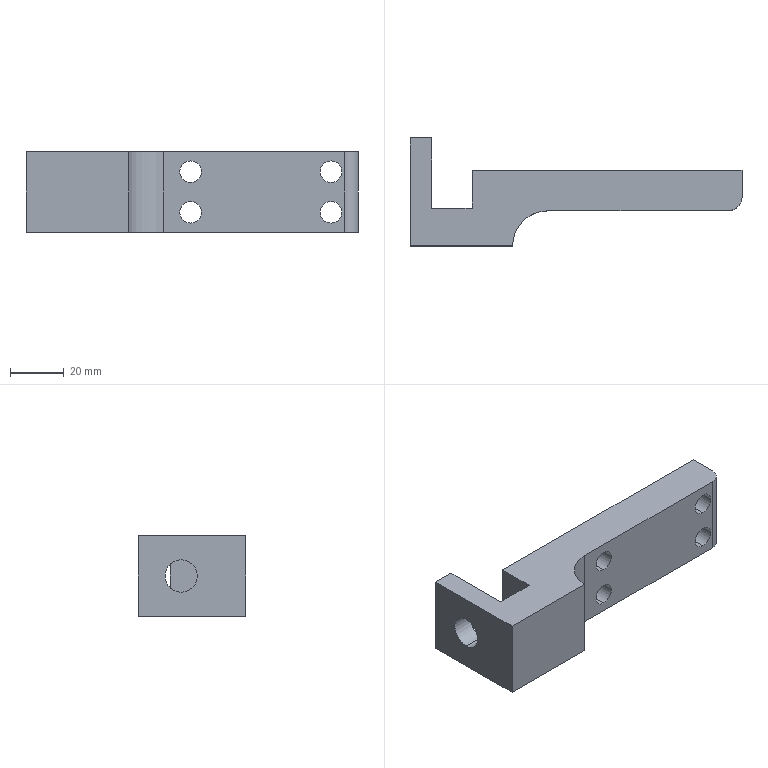Part | SolidWorks | features BaseBody 1 | 1 solid | 23 faces | box 123 x 40 x 30 mm | volume 63756 mm3 | cylinder 12 | plane 11 | commonest cylinder face diameters 8 x8 12 x2 10 x1 26 x1
STEP:
#1=CARTESIAN_POINT('',(340.,-80.,178.121));
#2=VERTEX_POINT('',#1);
#3=CARTESIAN_POINT('',(340.,-80.,186.121));
#4=VERTEX_POINT('',#3);
#5=CARTESIAN_POINT('',(340.,-80.,182.121));
#6=DIRECTION('',(0.,1.,0.));
#7=DIRECTION('',(0.,0.,-1.));
#8=AXIS2_PLACEMENT_3D('',#5,#6,#7);
#9=CIRCLE('',#8,4.);
#10=EDGE_CURVE('',#2,#4,#9,.T.);
#11=ORIENTED_EDGE('',*,*,#10,.T.);
#12=CARTESIAN_POINT('',(340.,-95.,186.121));
#13=VERTEX_POINT('',#12);
#14=CARTESIAN_POINT('',(340.,-95.,186.121));
#15=DIRECTION('',(0.,-1.,0.));
#16=VECTOR('',#15,1000.);
#17=LINE('',#14,#16);
#18=EDGE_CURVE('',#4,#13,#17,.T.);
#19=ORIENTED_EDGE('',*,*,#18,.T.);
#20=CARTESIAN_POINT('',(340.,-95.,178.121));
#21=VERTEX_POINT('',#20);
#22=CARTESIAN_POINT('',(340.,-95.,182.121));
#23=DIRECTION('',(0.,1.,0.));
#24=DIRECTION('',(0.,0.,-1.));
#25=AXIS2_PLACEMENT_3D('',#22,#23,#24);
#26=CIRCLE('',#25,4.);
#27=EDGE_CURVE('',#21,#13,#26,.T.);
#28=ORIENTED_EDGE('',*,*,#27,.F.);
#29=CARTESIAN_POINT('',(340.,-95.,178.121));
#30=DIRECTION('',(0.,-1.,0.));
#31=VECTOR('',#30,1000.);
#32=LINE('',#29,#31);
#33=EDGE_CURVE('',#2,#21,#32,.T.);
#34=ORIENTED_EDGE('',*,*,#33,.F.);
#35=EDGE_LOOP('',(#11,#19,#28,#34));
#36=FACE_OUTER_BOUND('',#35,.T.);
#37=CARTESIAN_POINT('',(340.,-95.,182.121));
#38=DIRECTION('',(0.,-1.,0.));
#39=DIRECTION('',(0.,0.,-1.));
#40=AXIS2_PLACEMENT_3D('',#37,#38,#39);
#41=CYLINDRICAL_SURFACE('',#40,4.);
#42=ADVANCED_FACE('',(#36),#41,.F.);
#43=CARTESIAN_POINT('',(340.,-80.,193.121));
#44=VERTEX_POINT('',#43);
#45=CARTESIAN_POINT('',(340.,-80.,201.121));
#46=VERTEX_POINT('',#45);
#47=CARTESIAN_POINT('',(340.,-80.,197.121));
#48=DIRECTION('',(0.,1.,0.));
#49=DIRECTION('',(0.,0.,-1.));
#50=AXIS2_PLACEMENT_3D('',#47,#48,#49);
#51=CIRCLE('',#50,4.);
#52=EDGE_CURVE('',#44,#46,#51,.T.);
#53=ORIENTED_EDGE('',*,*,#52,.T.);
#54=CARTESIAN_POINT('',(340.,-95.,201.121));
#55=VERTEX_POINT('',#54);
#56=CARTESIAN_POINT('',(340.,-95.,201.121));
#57=DIRECTION('',(0.,-1.,0.));
#58=VECTOR('',#57,1000.);
#59=LINE('',#56,#58);
#60=EDGE_CURVE('',#46,#55,#59,.T.);
#61=ORIENTED_EDGE('',*,*,#60,.T.);
#62=CARTESIAN_POINT('',(340.,-95.,193.121));
#63=VERTEX_POINT('',#62);
#64=CARTESIAN_POINT('',(340.,-95.,197.121));
#65=DIRECTION('',(0.,1.,0.));
#66=DIRECTION('',(0.,0.,-1.));
#67=AXIS2_PLACEMENT_3D('',#64,#65,#66);
#68=CIRCLE('',#67,4.);
#69=EDGE_CURVE('',#63,#55,#68,.T.);
#70=ORIENTED_EDGE('',*,*,#69,.F.);
#71=CARTESIAN_POINT('',(340.,-95.,193.121));
#72=DIRECTION('',(0.,-1.,0.));
#73=VECTOR('',#72,1000.);
#74=LINE('',#71,#73);
#75=EDGE_CURVE('',#44,#63,#74,.T.);
#76=ORIENTED_EDGE('',*,*,#75,.F.);
#77=EDGE_LOOP('',(#53,#61,#70,#76));
#78=FACE_OUTER_BOUND('',#77,.T.);
#79=CARTESIAN_POINT('',(340.,-95.,197.121));
#80=DIRECTION('',(0.,-1.,0.));
#81=DIRECTION('',(0.,0.,-1.));
#82=AXIS2_PLACEMENT_3D('',#79,#80,#81);
#83=CYLINDRICAL_SURFACE('',#82,4.);
#84=ADVANCED_FACE('',(#78),#83,.F.);
#85=CARTESIAN_POINT('',(288.,-80.,193.121));
#86=VERTEX_POINT('',#85);
#87=CARTESIAN_POINT('',(288.,-80.,201.121));
#88=VERTEX_POINT('',#87);
#89=CARTESIAN_POINT('',(288.,-80.,197.121));
#90=DIRECTION('',(0.,1.,0.));
#91=DIRECTION('',(0.,0.,-1.));
#92=AXIS2_PLACEMENT_3D('',#89,#90,#91);
#93=CIRCLE('',#92,4.);
#94=EDGE_CURVE('',#86,#88,#93,.T.);
#95=ORIENTED_EDGE('',*,*,#94,.T.);
#96=CARTESIAN_POINT('',(288.,-95.,201.121));
#97=VERTEX_POINT('',#96);
#98=CARTESIAN_POINT('',(288.,-95.,201.121));
#99=DIRECTION('',(0.,-1.,0.));
#100=VECTOR('',#99,1000.);
#101=LINE('',#98,#100);
#102=EDGE_CURVE('',#88,#97,#101,.T.);
#103=ORIENTED_EDGE('',*,*,#102,.T.);
#104=CARTESIAN_POINT('',(288.,-95.,193.121));
#105=VERTEX_POINT('',#104);
#106=CARTESIAN_POINT('',(288.,-95.,197.121));
#107=DIRECTION('',(0.,1.,0.));
#108=DIRECTION('',(0.,0.,-1.));
#109=AXIS2_PLACEMENT_3D('',#106,#107,#108);
#110=CIRCLE('',#109,4.);
#111=EDGE_CURVE('',#105,#97,#110,.T.);
#112=ORIENTED_EDGE('',*,*,#111,.F.);
#113=CARTESIAN_POINT('',(288.,-95.,193.121));
#114=DIRECTION('',(0.,-1.,0.));
#115=VECTOR('',#114,1000.);
#116=LINE('',#113,#115);
#117=EDGE_CURVE('',#86,#105,#116,.T.);
#118=ORIENTED_EDGE('',*,*,#117,.F.);
#119=EDGE_LOOP('',(#95,#103,#112,#118));
#120=FACE_OUTER_BOUND('',#119,.T.);
#121=CARTESIAN_POINT('',(288.,-95.,197.121));
#122=DIRECTION('',(0.,-1.,0.));
#123=DIRECTION('',(0.,0.,-1.));
#124=AXIS2_PLACEMENT_3D('',#121,#122,#123);
#125=CYLINDRICAL_SURFACE('',#124,4.);
#126=ADVANCED_FACE('',(#120),#125,.F.);
#127=CARTESIAN_POINT('',(288.,-80.,178.121));
#128=VERTEX_POINT('',#127);
#129=CARTESIAN_POINT('',(288.,-80.,186.121));
#130=VERTEX_POINT('',#129);
#131=CARTESIAN_POINT('',(288.,-80.,182.121));
#132=DIRECTION('',(0.,1.,0.));
#133=DIRECTION('',(0.,0.,-1.));
#134=AXIS2_PLACEMENT_3D('',#131,#132,#133);
#135=CIRCLE('',#134,4.);
#136=EDGE_CURVE('',#128,#130,#135,.T.);
#137=ORIENTED_EDGE('',*,*,#136,.T.);
#138=CARTESIAN_POINT('',(288.,-95.,186.121));
#139=VERTEX_POINT('',#138);
#140=CARTESIAN_POINT('',(288.,-95.,186.121));
#141=DIRECTION('',(0.,-1.,0.));
#142=VECTOR('',#141,1000.);
#143=LINE('',#140,#142);
#144=EDGE_CURVE('',#130,#139,#143,.T.);
#145=ORIENTED_EDGE('',*,*,#144,.T.);
#146=CARTESIAN_POINT('',(288.,-95.,178.121));
#147=VERTEX_POINT('',#146);
#148=CARTESIAN_POINT('',(288.,-95.,182.121));
#149=DIRECTION('',(0.,1.,0.));
#150=DIRECTION('',(0.,0.,-1.));
#151=AXIS2_PLACEMENT_3D('',#148,#149,#150);
#152=CIRCLE('',#151,4.);
#153=EDGE_CURVE('',#147,#139,#152,.T.);
#154=ORIENTED_EDGE('',*,*,#153,.F.);
#155=CARTESIAN_POINT('',(288.,-95.,178.121));
#156=DIRECTION('',(0.,-1.,0.));
#157=VECTOR('',#156,1000.);
#158=LINE('',#155,#157);
#159=EDGE_CURVE('',#128,#147,#158,.T.);
#160=ORIENTED_EDGE('',*,*,#159,.F.);
#161=EDGE_LOOP('',(#137,#145,#154,#160));
#162=FACE_OUTER_BOUND('',#161,.T.);
#163=CARTESIAN_POINT('',(288.,-95.,182.121));
#164=DIRECTION('',(0.,-1.,0.));
#165=DIRECTION('',(0.,0.,-1.));
#166=AXIS2_PLACEMENT_3D('',#163,#164,#165);
#167=CYLINDRICAL_SURFACE('',#166,4.);
#168=ADVANCED_FACE('',(#162),#167,.F.);
#169=CARTESIAN_POINT('',(235.,-84.,195.621));
#170=VERTEX_POINT('',#169);
#171=CARTESIAN_POINT('',(235.,-84.,183.621));
#172=VERTEX_POINT('',#171);
#173=CARTESIAN_POINT('',(235.,-84.,189.621));
#174=DIRECTION('',(1.,0.,0.));
#175=DIRECTION('',(0.,0.,1.));
#176=AXIS2_PLACEMENT_3D('',#173,#174,#175);
#177=CIRCLE('',#176,6.);
#178=EDGE_CURVE('',#170,#172,#177,.T.);
#179=ORIENTED_EDGE('',*,*,#178,.T.);
#180=CARTESIAN_POINT('',(227.,-84.,183.621));
#181=VERTEX_POINT('',#180);
#182=CARTESIAN_POINT('',(251.971,-84.,183.621));
#183=DIRECTION('',(-1.,0.,0.));
#184=VECTOR('',#183,1000.);
#185=LINE('',#182,#184);
#186=EDGE_CURVE('',#172,#181,#185,.T.);
#187=ORIENTED_EDGE('',*,*,#186,.T.);
#188=CARTESIAN_POINT('',(227.,-84.,195.621));
#189=VERTEX_POINT('',#188);
#190=CARTESIAN_POINT('',(227.,-84.,189.621));
#191=DIRECTION('',(-1.,0.,0.));
#192=DIRECTION('',(0.,0.,1.));
#193=AXIS2_PLACEMENT_3D('',#190,#191,#192);
#194=CIRCLE('',#193,6.);
#195=EDGE_CURVE('',#181,#189,#194,.T.);
#196=ORIENTED_EDGE('',*,*,#195,.T.);
#197=CARTESIAN_POINT('',(251.971,-84.,195.621));
#198=DIRECTION('',(-1.,0.,0.));
#199=VECTOR('',#198,1000.);
#200=LINE('',#197,#199);
#201=EDGE_CURVE('',#170,#189,#200,.T.);
#202=ORIENTED_EDGE('',*,*,#201,.F.);
#203=EDGE_LOOP('',(#179,#187,#196,#202));
#204=FACE_OUTER_BOUND('',#203,.T.);
#205=CARTESIAN_POINT('',(251.971,-84.,189.621));
#206=DIRECTION('',(-1.,0.,0.));
#207=DIRECTION('',(0.,0.,1.));
#208=AXIS2_PLACEMENT_3D('',#205,#206,#207);
#209=CYLINDRICAL_SURFACE('',#208,6.);
#210=ADVANCED_FACE('',(#204),#209,.F.);
#211=CARTESIAN_POINT('',(350.,-80.,174.621));
#212=VERTEX_POINT('',#211);
#213=CARTESIAN_POINT('',(350.,-80.,204.621));
#214=VERTEX_POINT('',#213);
#215=CARTESIAN_POINT('',(350.,-80.,174.621));
#216=DIRECTION('',(0.,0.,1.));
#217=VECTOR('',#216,1000.);
#218=LINE('',#215,#217);
#219=EDGE_CURVE('',#212,#214,#218,.T.);
#220=ORIENTED_EDGE('',*,*,#219,.F.);
#221=CARTESIAN_POINT('',(250.,-80.,174.621));
#222=VERTEX_POINT('',#221);
#223=CARTESIAN_POINT('',(350.,-80.,174.621));
#224=DIRECTION('',(1.,0.,0.));
#225=VECTOR('',#224,1000.);
#226=LINE('',#223,#225);
#227=EDGE_CURVE('',#222,#212,#226,.T.);
#228=ORIENTED_EDGE('',*,*,#227,.F.);
#229=CARTESIAN_POINT('',(250.,-80.,204.621));
#230=VERTEX_POINT('',#229);
#231=CARTESIAN_POINT('',(250.,-80.,174.621));
#232=DIRECTION('',(0.,0.,-1.));
#233=VECTOR('',#232,1000.);
#234=LINE('',#231,#233);
#235=EDGE_CURVE('',#230,#222,#234,.T.);
#236=ORIENTED_EDGE('',*,*,#235,.F.);
#237=CARTESIAN_POINT('',(350.,-80.,204.621));
#238=DIRECTION('',(-1.,0.,0.));
#239=VECTOR('',#238,1000.);
#240=LINE('',#237,#239);
#241=EDGE_CURVE('',#214,#230,#240,.T.);
#242=ORIENTED_EDGE('',*,*,#241,.F.);
#243=EDGE_LOOP('',(#220,#228,#236,#242));
#244=FACE_OUTER_BOUND('',#243,.T.);
#245=ORIENTED_EDGE('',*,*,#10,.F.);
#246=CARTESIAN_POINT('',(340.,-80.,182.121));
#247=DIRECTION('',(0.,1.,0.));
#248=DIRECTION('',(0.,0.,-1.));
#249=AXIS2_PLACEMENT_3D('',#246,#247,#248);
#250=CIRCLE('',#249,4.);
#251=EDGE_CURVE('',#4,#2,#250,.T.);
#252=ORIENTED_EDGE('',*,*,#251,.F.);
#253=EDGE_LOOP('',(#245,#252));
#254=FACE_BOUND('',#253,.T.);
#255=ORIENTED_EDGE('',*,*,#52,.F.);
#256=CARTESIAN_POINT('',(340.,-80.,197.121));
#257=DIRECTION('',(0.,1.,0.));
#258=DIRECTION('',(0.,0.,-1.));
#259=AXIS2_PLACEMENT_3D('',#256,#257,#258);
#260=CIRCLE('',#259,4.);
#261=EDGE_CURVE('',#46,#44,#260,.T.);
#262=ORIENTED_EDGE('',*,*,#261,.F.);
#263=EDGE_LOOP('',(#255,#262));
#264=FACE_BOUND('',#263,.T.);
#265=ORIENTED_EDGE('',*,*,#94,.F.);
#266=CARTESIAN_POINT('',(288.,-80.,197.121));
#267=DIRECTION('',(0.,1.,0.));
#268=DIRECTION('',(0.,0.,-1.));
#269=AXIS2_PLACEMENT_3D('',#266,#267,#268);
#270=CIRCLE('',#269,4.);
#271=EDGE_CURVE('',#88,#86,#270,.T.);
#272=ORIENTED_EDGE('',*,*,#271,.F.);
#273=EDGE_LOOP('',(#265,#272));
#274=FACE_BOUND('',#273,.T.);
#275=ORIENTED_EDGE('',*,*,#136,.F.);
#276=CARTESIAN_POINT('',(288.,-80.,182.121));
#277=DIRECTION('',(0.,1.,0.));
#278=DIRECTION('',(0.,0.,-1.));
#279=AXIS2_PLACEMENT_3D('',#276,#277,#278);
#280=CIRCLE('',#279,4.);
#281=EDGE_CURVE('',#130,#128,#280,.T.);
#282=ORIENTED_EDGE('',*,*,#281,.F.);
#283=EDGE_LOOP('',(#275,#282));
#284=FACE_BOUND('',#283,.T.);
#285=CARTESIAN_POINT('',(350.,-80.,174.621));
#286=DIRECTION('',(0.,-1.,0.));
#287=DIRECTION('',(0.,0.,-1.));
#288=AXIS2_PLACEMENT_3D('',#285,#286,#287);
#289=PLANE('',#288);
#290=ADVANCED_FACE('',(#244,#254,#264,#274,#284),#289,.F.);
#291=CARTESIAN_POINT('',(350.,-90.,204.621));
#292=VERTEX_POINT('',#291);
#293=CARTESIAN_POINT('',(345.,-95.,204.621));
#294=VERTEX_POINT('',#293);
#295=CARTESIAN_POINT('',(345.,-90.,204.621));
#296=DIRECTION('',(0.,0.,-1.));
#297=DIRECTION('',(1.,0.,0.));
#298=AXIS2_PLACEMENT_3D('',#295,#296,#297);
#299=CIRCLE('',#298,5.);
#300=EDGE_CURVE('',#292,#294,#299,.T.);
#301=ORIENTED_EDGE('',*,*,#300,.F.);
#302=CARTESIAN_POINT('',(350.,-82.6,204.621));
#303=DIRECTION('',(0.,-1.,0.));
#304=VECTOR('',#303,1000.);
#305=LINE('',#302,#304);
#306=EDGE_CURVE('',#214,#292,#305,.T.);
#307=ORIENTED_EDGE('',*,*,#306,.F.);
#308=ORIENTED_EDGE('',*,*,#241,.T.);
#309=CARTESIAN_POINT('',(250.,-94.,204.621));
#310=VERTEX_POINT('',#309);
#311=CARTESIAN_POINT('',(250.,-82.6,204.621));
#312=DIRECTION('',(0.,1.,0.));
#313=VECTOR('',#312,1000.);
#314=LINE('',#311,#313);
#315=EDGE_CURVE('',#310,#230,#314,.T.);
#316=ORIENTED_EDGE('',*,*,#315,.F.);
#317=CARTESIAN_POINT('',(235.,-94.,204.621));
#318=VERTEX_POINT('',#317);
#319=CARTESIAN_POINT('',(251.867,-94.,204.621));
#320=DIRECTION('',(1.,0.,0.));
#321=VECTOR('',#320,1000.);
#322=LINE('',#319,#321);
#323=EDGE_CURVE('',#318,#310,#322,.T.);
#324=ORIENTED_EDGE('',*,*,#323,.F.);
#325=CARTESIAN_POINT('',(235.,-68.,204.621));
#326=VERTEX_POINT('',#325);
#327=CARTESIAN_POINT('',(235.,-82.6,204.621));
#328=DIRECTION('',(0.,-1.,0.));
#329=VECTOR('',#328,1000.);
#330=LINE('',#327,#329);
#331=EDGE_CURVE('',#326,#318,#330,.T.);
#332=ORIENTED_EDGE('',*,*,#331,.F.);
#333=CARTESIAN_POINT('',(227.,-68.,204.621));
#334=VERTEX_POINT('',#333);
#335=CARTESIAN_POINT('',(251.867,-68.,204.621));
#336=DIRECTION('',(1.,0.,0.));
#337=VECTOR('',#336,1000.);
#338=LINE('',#335,#337);
#339=EDGE_CURVE('',#334,#326,#338,.T.);
#340=ORIENTED_EDGE('',*,*,#339,.F.);
#341=CARTESIAN_POINT('',(227.,-108.,204.621));
#342=VERTEX_POINT('',#341);
#343=CARTESIAN_POINT('',(227.,-82.6,204.621));
#344=DIRECTION('',(0.,1.,0.));
#345=VECTOR('',#344,1000.);
#346=LINE('',#343,#345);
#347=EDGE_CURVE('',#342,#334,#346,.T.);
#348=ORIENTED_EDGE('',*,*,#347,.F.);
#349=CARTESIAN_POINT('',(265.,-108.,204.621));
#350=VERTEX_POINT('',#349);
#351=CARTESIAN_POINT('',(251.867,-108.,204.621));
#352=DIRECTION('',(-1.,0.,0.));
#353=VECTOR('',#352,1000.);
#354=LINE('',#351,#353);
#355=EDGE_CURVE('',#350,#342,#354,.T.);
#356=ORIENTED_EDGE('',*,*,#355,.F.);
#357=CARTESIAN_POINT('',(278.,-95.,204.621));
#358=VERTEX_POINT('',#357);
#359=CARTESIAN_POINT('',(278.,-108.,204.621));
#360=DIRECTION('',(0.,0.,1.));
#361=DIRECTION('',(-1.,0.,0.));
#362=AXIS2_PLACEMENT_3D('',#359,#360,#361);
#363=CIRCLE('',#362,13.);
#364=EDGE_CURVE('',#358,#350,#363,.T.);
#365=ORIENTED_EDGE('',*,*,#364,.F.);
#366=CARTESIAN_POINT('',(251.867,-95.,204.621));
#367=DIRECTION('',(-1.,0.,0.));
#368=VECTOR('',#367,1000.);
#369=LINE('',#366,#368);
#370=EDGE_CURVE('',#294,#358,#369,.T.);
#371=ORIENTED_EDGE('',*,*,#370,.F.);
#372=EDGE_LOOP('',(#301,#307,#308,#316,#324,#332,#340,#348,#356,#365,#371));
#373=FACE_OUTER_BOUND('',#372,.T.);
#374=CARTESIAN_POINT('',(251.867,-82.6,204.621));
#375=DIRECTION('',(0.,0.,-1.));
#376=DIRECTION('',(-1.,0.,0.));
#377=AXIS2_PLACEMENT_3D('',#374,#375,#376);
#378=PLANE('',#377);
#379=ADVANCED_FACE('',(#373),#378,.F.);
#380=CARTESIAN_POINT('',(350.,-90.,174.621));
#381=VERTEX_POINT('',#380);
#382=CARTESIAN_POINT('',(350.,-90.,174.621));
#383=DIRECTION('',(0.,0.,1.));
#384=VECTOR('',#383,1000.);
#385=LINE('',#382,#384);
#386=EDGE_CURVE('',#381,#292,#385,.T.);
#387=ORIENTED_EDGE('',*,*,#386,.F.);
#388=CARTESIAN_POINT('',(350.,-80.,174.621));
#389=DIRECTION('',(0.,-1.,0.));
#390=VECTOR('',#389,1000.);
#391=LINE('',#388,#390);
#392=EDGE_CURVE('',#212,#381,#391,.T.);
#393=ORIENTED_EDGE('',*,*,#392,.F.);
#394=ORIENTED_EDGE('',*,*,#219,.T.);
#395=ORIENTED_EDGE('',*,*,#306,.T.);
#396=EDGE_LOOP('',(#387,#393,#394,#395));
#397=FACE_OUTER_BOUND('',#396,.T.);
#398=CARTESIAN_POINT('',(350.,-80.,174.621));
#399=DIRECTION('',(-1.,0.,0.));
#400=DIRECTION('',(0.,0.,1.));
#401=AXIS2_PLACEMENT_3D('',#398,#399,#400);
#402=PLANE('',#401);
#403=ADVANCED_FACE('',(#397),#402,.F.);
#404=CARTESIAN_POINT('',(250.,-94.,174.621));
#405=VERTEX_POINT('',#404);
#406=CARTESIAN_POINT('',(250.,-82.6,174.621));
#407=DIRECTION('',(0.,1.,0.));
#408=VECTOR('',#407,1000.);
#409=LINE('',#406,#408);
#410=EDGE_CURVE('',#405,#222,#409,.T.);
#411=ORIENTED_EDGE('',*,*,#410,.T.);
#412=ORIENTED_EDGE('',*,*,#227,.T.);
#413=ORIENTED_EDGE('',*,*,#392,.T.);
#414=CARTESIAN_POINT('',(345.,-95.,174.621));
#415=VERTEX_POINT('',#414);
#416=CARTESIAN_POINT('',(345.,-90.,174.621));
#417=DIRECTION('',(0.,0.,-1.));
#418=DIRECTION('',(1.,0.,0.));
#419=AXIS2_PLACEMENT_3D('',#416,#417,#418);
#420=CIRCLE('',#419,5.);
#421=EDGE_CURVE('',#381,#415,#420,.T.);
#422=ORIENTED_EDGE('',*,*,#421,.T.);
#423=CARTESIAN_POINT('',(278.,-95.,174.621));
#424=VERTEX_POINT('',#423);
#425=CARTESIAN_POINT('',(251.867,-95.,174.621));
#426=DIRECTION('',(-1.,0.,0.));
#427=VECTOR('',#426,1000.);
#428=LINE('',#425,#427);
#429=EDGE_CURVE('',#415,#424,#428,.T.);
#430=ORIENTED_EDGE('',*,*,#429,.T.);
#431=CARTESIAN_POINT('',(265.,-108.,174.621));
#432=VERTEX_POINT('',#431);
#433=CARTESIAN_POINT('',(278.,-108.,174.621));
#434=DIRECTION('',(0.,0.,1.));
#435=DIRECTION('',(-1.,0.,0.));
#436=AXIS2_PLACEMENT_3D('',#433,#434,#435);
#437=CIRCLE('',#436,13.);
#438=EDGE_CURVE('',#424,#432,#437,.T.);
#439=ORIENTED_EDGE('',*,*,#438,.T.);
#440=CARTESIAN_POINT('',(227.,-108.,174.621));
#441=VERTEX_POINT('',#440);
#442=CARTESIAN_POINT('',(251.867,-108.,174.621));
#443=DIRECTION('',(-1.,0.,0.));
#444=VECTOR('',#443,1000.);
#445=LINE('',#442,#444);
#446=EDGE_CURVE('',#432,#441,#445,.T.);
#447=ORIENTED_EDGE('',*,*,#446,.T.);
#448=CARTESIAN_POINT('',(227.,-68.,174.621));
#449=VERTEX_POINT('',#448);
#450=CARTESIAN_POINT('',(227.,-82.6,174.621));
#451=DIRECTION('',(0.,1.,0.));
#452=VECTOR('',#451,1000.);
#453=LINE('',#450,#452);
#454=EDGE_CURVE('',#441,#449,#453,.T.);
#455=ORIENTED_EDGE('',*,*,#454,.T.);
#456=CARTESIAN_POINT('',(235.,-68.,174.621));
#457=VERTEX_POINT('',#456);
#458=CARTESIAN_POINT('',(251.867,-68.,174.621));
#459=DIRECTION('',(1.,0.,0.));
#460=VECTOR('',#459,1000.);
#461=LINE('',#458,#460);
#462=EDGE_CURVE('',#449,#457,#461,.T.);
#463=ORIENTED_EDGE('',*,*,#462,.T.);
#464=CARTESIAN_POINT('',(235.,-94.,174.621));
#465=VERTEX_POINT('',#464);
#466=CARTESIAN_POINT('',(235.,-82.6,174.621));
#467=DIRECTION('',(0.,-1.,0.));
#468=VECTOR('',#467,1000.);
#469=LINE('',#466,#468);
#470=EDGE_CURVE('',#457,#465,#469,.T.);
#471=ORIENTED_EDGE('',*,*,#470,.T.);
#472=CARTESIAN_POINT('',(251.867,-94.,174.621));
#473=DIRECTION('',(1.,0.,0.));
#474=VECTOR('',#473,1000.);
#475=LINE('',#472,#474);
#476=EDGE_CURVE('',#465,#405,#475,.T.);
#477=ORIENTED_EDGE('',*,*,#476,.T.);
#478=EDGE_LOOP('',(#411,#412,#413,#422,#430,#439,#447,#455,#463,#471,#477));
#479=FACE_OUTER_BOUND('',#478,.T.);
#480=CARTESIAN_POINT('',(251.867,-82.6,174.621));
#481=DIRECTION('',(0.,0.,-1.));
#482=DIRECTION('',(-1.,0.,0.));
#483=AXIS2_PLACEMENT_3D('',#480,#481,#482);
#484=PLANE('',#483);
#485=ADVANCED_FACE('',(#479),#484,.T.);
#486=ORIENTED_EDGE('',*,*,#235,.T.);
#487=ORIENTED_EDGE('',*,*,#410,.F.);
#488=CARTESIAN_POINT('',(250.,-94.,174.621));
#489=DIRECTION('',(0.,0.,-1.));
#490=VECTOR('',#489,1000.);
#491=LINE('',#488,#490);
#492=EDGE_CURVE('',#310,#405,#491,.T.);
#493=ORIENTED_EDGE('',*,*,#492,.F.);
#494=ORIENTED_EDGE('',*,*,#315,.T.);
#495=EDGE_LOOP('',(#486,#487,#493,#494));
#496=FACE_OUTER_BOUND('',#495,.T.);
#497=CARTESIAN_POINT('',(250.,-80.,174.621));
#498=DIRECTION('',(1.,0.,0.));
#499=DIRECTION('',(0.,0.,-1.));
#500=AXIS2_PLACEMENT_3D('',#497,#498,#499);
#501=PLANE('',#500);
#502=ADVANCED_FACE('',(#496),#501,.F.);
#503=ORIENTED_EDGE('',*,*,#18,.F.);
#504=ORIENTED_EDGE('',*,*,#251,.T.);
#505=ORIENTED_EDGE('',*,*,#33,.T.);
#506=CARTESIAN_POINT('',(340.,-95.,182.121));
#507=DIRECTION('',(0.,1.,0.));
#508=DIRECTION('',(0.,0.,-1.));
#509=AXIS2_PLACEMENT_3D('',#506,#507,#508);
#510=CIRCLE('',#509,4.);
#511=EDGE_CURVE('',#13,#21,#510,.T.);
#512=ORIENTED_EDGE('',*,*,#511,.F.);
#513=EDGE_LOOP('',(#503,#504,#505,#512));
#514=FACE_OUTER_BOUND('',#513,.T.);
#515=CARTESIAN_POINT('',(340.,-95.,182.121));
#516=DIRECTION('',(0.,-1.,0.));
#517=DIRECTION('',(0.,0.,-1.));
#518=AXIS2_PLACEMENT_3D('',#515,#516,#517);
#519=CYLINDRICAL_SURFACE('',#518,4.);
#520=ADVANCED_FACE('',(#514),#519,.F.);
#521=ORIENTED_EDGE('',*,*,#60,.F.);
#522=ORIENTED_EDGE('',*,*,#261,.T.);
#523=ORIENTED_EDGE('',*,*,#75,.T.);
#524=CARTESIAN_POINT('',(340.,-95.,197.121));
#525=DIRECTION('',(0.,1.,0.));
#526=DIRECTION('',(0.,0.,-1.));
#527=AXIS2_PLACEMENT_3D('',#524,#525,#526);
#528=CIRCLE('',#527,4.);
#529=EDGE_CURVE('',#55,#63,#528,.T.);
#530=ORIENTED_EDGE('',*,*,#529,.F.);
#531=EDGE_LOOP('',(#521,#522,#523,#530));
#532=FACE_OUTER_BOUND('',#531,.T.);
#533=CARTESIAN_POINT('',(340.,-95.,197.121));
#534=DIRECTION('',(0.,-1.,0.));
#535=DIRECTION('',(0.,0.,-1.));
#536=AXIS2_PLACEMENT_3D('',#533,#534,#535);
#537=CYLINDRICAL_SURFACE('',#536,4.);
#538=ADVANCED_FACE('',(#532),#537,.F.);
#539=ORIENTED_EDGE('',*,*,#102,.F.);
#540=ORIENTED_EDGE('',*,*,#271,.T.);
#541=ORIENTED_EDGE('',*,*,#117,.T.);
#542=CARTESIAN_POINT('',(288.,-95.,197.121));
#543=DIRECTION('',(0.,1.,0.));
#544=DIRECTION('',(0.,0.,-1.));
#545=AXIS2_PLACEMENT_3D('',#542,#543,#544);
#546=CIRCLE('',#545,4.);
#547=EDGE_CURVE('',#97,#105,#546,.T.);
#548=ORIENTED_EDGE('',*,*,#547,.F.);
#549=EDGE_LOOP('',(#539,#540,#541,#548));
#550=FACE_OUTER_BOUND('',#549,.T.);
#551=CARTESIAN_POINT('',(288.,-95.,197.121));
#552=DIRECTION('',(0.,-1.,0.));
#553=DIRECTION('',(0.,0.,-1.));
#554=AXIS2_PLACEMENT_3D('',#551,#552,#553);
#555=CYLINDRICAL_SURFACE('',#554,4.);
#556=ADVANCED_FACE('',(#550),#555,.F.);
#557=ORIENTED_EDGE('',*,*,#144,.F.);
#558=ORIENTED_EDGE('',*,*,#281,.T.);
#559=ORIENTED_EDGE('',*,*,#159,.T.);
#560=CARTESIAN_POINT('',(288.,-95.,182.121));
#561=DIRECTION('',(0.,1.,0.));
#562=DIRECTION('',(0.,0.,-1.));
#563=AXIS2_PLACEMENT_3D('',#560,#561,#562);
#564=CIRCLE('',#563,4.);
#565=EDGE_CURVE('',#139,#147,#564,.T.);
#566=ORIENTED_EDGE('',*,*,#565,.F.);
#567=EDGE_LOOP('',(#557,#558,#559,#566));
#568=FACE_OUTER_BOUND('',#567,.T.);
#569=CARTESIAN_POINT('',(288.,-95.,182.121));
#570=DIRECTION('',(0.,-1.,0.));
#571=DIRECTION('',(0.,0.,-1.));
#572=AXIS2_PLACEMENT_3D('',#569,#570,#571);
#573=CYLINDRICAL_SURFACE('',#572,4.);
#574=ADVANCED_FACE('',(#568),#573,.F.);
#575=CARTESIAN_POINT('',(345.,-95.,174.621));
#576=DIRECTION('',(0.,0.,-1.));
#577=VECTOR('',#576,1000.);
#578=LINE('',#575,#577);
#579=EDGE_CURVE('',#294,#415,#578,.T.);
#580=ORIENTED_EDGE('',*,*,#579,.F.);
#581=ORIENTED_EDGE('',*,*,#370,.T.);
#582=CARTESIAN_POINT('',(278.,-95.,174.621));
#583=DIRECTION('',(0.,0.,1.));
#584=VECTOR('',#583,1000.);
#585=LINE('',#582,#584);
#586=EDGE_CURVE('',#424,#358,#585,.T.);
#587=ORIENTED_EDGE('',*,*,#586,.F.);
#588=ORIENTED_EDGE('',*,*,#429,.F.);
#589=EDGE_LOOP('',(#580,#581,#587,#588));
#590=FACE_OUTER_BOUND('',#589,.T.);
#591=ORIENTED_EDGE('',*,*,#27,.T.);
#592=ORIENTED_EDGE('',*,*,#511,.T.);
#593=EDGE_LOOP('',(#591,#592));
#594=FACE_BOUND('',#593,.T.);
#595=ORIENTED_EDGE('',*,*,#69,.T.);
#596=ORIENTED_EDGE('',*,*,#529,.T.);
#597=EDGE_LOOP('',(#595,#596));
#598=FACE_BOUND('',#597,.T.);
#599=ORIENTED_EDGE('',*,*,#111,.T.);
#600=ORIENTED_EDGE('',*,*,#547,.T.);
#601=EDGE_LOOP('',(#599,#600));
#602=FACE_BOUND('',#601,.T.);
#603=ORIENTED_EDGE('',*,*,#153,.T.);
#604=ORIENTED_EDGE('',*,*,#565,.T.);
#605=EDGE_LOOP('',(#603,#604));
#606=FACE_BOUND('',#605,.T.);
#607=CARTESIAN_POINT('',(350.,-95.,174.621));
#608=DIRECTION('',(0.,1.,0.));
#609=DIRECTION('',(0.,0.,1.));
#610=AXIS2_PLACEMENT_3D('',#607,#608,#609);
#611=PLANE('',#610);
#612=ADVANCED_FACE('',(#590,#594,#598,#602,#606),#611,.F.);
#613=ORIENTED_EDGE('',*,*,#300,.T.);
#614=ORIENTED_EDGE('',*,*,#579,.T.);
#615=ORIENTED_EDGE('',*,*,#421,.F.);
#616=ORIENTED_EDGE('',*,*,#386,.T.);
#617=EDGE_LOOP('',(#613,#614,#615,#616));
#618=FACE_OUTER_BOUND('',#617,.T.);
#619=CARTESIAN_POINT('',(345.,-90.,174.621));
#620=DIRECTION('',(0.,0.,1.));
#621=DIRECTION('',(1.,0.,0.));
#622=AXIS2_PLACEMENT_3D('',#619,#620,#621);
#623=CYLINDRICAL_SURFACE('',#622,5.);
#624=ADVANCED_FACE('',(#618),#623,.T.);
#625=ORIENTED_EDGE('',*,*,#492,.T.);
#626=ORIENTED_EDGE('',*,*,#476,.F.);
#627=CARTESIAN_POINT('',(235.,-94.,174.621));
#628=DIRECTION('',(0.,0.,-1.));
#629=VECTOR('',#628,1000.);
#630=LINE('',#627,#629);
#631=EDGE_CURVE('',#318,#465,#630,.T.);
#632=ORIENTED_EDGE('',*,*,#631,.F.);
#633=ORIENTED_EDGE('',*,*,#323,.T.);
#634=EDGE_LOOP('',(#625,#626,#632,#633));
#635=FACE_OUTER_BOUND('',#634,.T.);
#636=CARTESIAN_POINT('',(250.,-94.,174.621));
#637=DIRECTION('',(0.,-1.,0.));
#638=DIRECTION('',(0.,0.,-1.));
#639=AXIS2_PLACEMENT_3D('',#636,#637,#638);
#640=PLANE('',#639);
#641=ADVANCED_FACE('',(#635),#640,.F.);
#642=ORIENTED_EDGE('',*,*,#631,.T.);
#643=ORIENTED_EDGE('',*,*,#470,.F.);
#644=CARTESIAN_POINT('',(235.,-68.,174.621));
#645=DIRECTION('',(0.,0.,-1.));
#646=VECTOR('',#645,1000.);
#647=LINE('',#644,#646);
#648=EDGE_CURVE('',#326,#457,#647,.T.);
#649=ORIENTED_EDGE('',*,*,#648,.F.);
#650=ORIENTED_EDGE('',*,*,#331,.T.);
#651=EDGE_LOOP('',(#642,#643,#649,#650));
#652=FACE_OUTER_BOUND('',#651,.T.);
#653=ORIENTED_EDGE('',*,*,#178,.F.);
#654=CARTESIAN_POINT('',(235.,-84.,189.621));
#655=DIRECTION('',(1.,0.,0.));
#656=DIRECTION('',(0.,0.,1.));
#657=AXIS2_PLACEMENT_3D('',#654,#655,#656);
#658=CIRCLE('',#657,6.);
#659=EDGE_CURVE('',#172,#170,#658,.T.);
#660=ORIENTED_EDGE('',*,*,#659,.F.);
#661=EDGE_LOOP('',(#653,#660));
#662=FACE_BOUND('',#661,.T.);
#663=CARTESIAN_POINT('',(235.,-94.,174.621));
#664=DIRECTION('',(-1.,0.,0.));
#665=DIRECTION('',(0.,0.,1.));
#666=AXIS2_PLACEMENT_3D('',#663,#664,#665);
#667=PLANE('',#666);
#668=ADVANCED_FACE('',(#652,#662),#667,.F.);
#669=ORIENTED_EDGE('',*,*,#648,.T.);
#670=ORIENTED_EDGE('',*,*,#462,.F.);
#671=CARTESIAN_POINT('',(227.,-68.,174.621));
#672=DIRECTION('',(0.,0.,-1.));
#673=VECTOR('',#672,1000.);
#674=LINE('',#671,#673);
#675=EDGE_CURVE('',#334,#449,#674,.T.);
#676=ORIENTED_EDGE('',*,*,#675,.F.);
#677=ORIENTED_EDGE('',*,*,#339,.T.);
#678=EDGE_LOOP('',(#669,#670,#676,#677));
#679=FACE_OUTER_BOUND('',#678,.T.);
#680=CARTESIAN_POINT('',(227.,-68.,174.621));
#681=DIRECTION('',(0.,-1.,0.));
#682=DIRECTION('',(0.,0.,-1.));
#683=AXIS2_PLACEMENT_3D('',#680,#681,#682);
#684=PLANE('',#683);
#685=ADVANCED_FACE('',(#679),#684,.F.);
#686=ORIENTED_EDGE('',*,*,#675,.T.);
#687=ORIENTED_EDGE('',*,*,#454,.F.);
#688=CARTESIAN_POINT('',(227.,-108.,174.621));
#689=DIRECTION('',(0.,0.,-1.));
#690=VECTOR('',#689,1000.);
#691=LINE('',#688,#690);
#692=EDGE_CURVE('',#342,#441,#691,.T.);
#693=ORIENTED_EDGE('',*,*,#692,.F.);
#694=ORIENTED_EDGE('',*,*,#347,.T.);
#695=EDGE_LOOP('',(#686,#687,#693,#694));
#696=FACE_OUTER_BOUND('',#695,.T.);
#697=CARTESIAN_POINT('',(227.,-84.,189.621));
#698=DIRECTION('',(-1.,0.,0.));
#699=DIRECTION('',(0.,0.,1.));
#700=AXIS2_PLACEMENT_3D('',#697,#698,#699);
#701=CIRCLE('',#700,6.);
#702=EDGE_CURVE('',#189,#181,#701,.T.);
#703=ORIENTED_EDGE('',*,*,#702,.F.);
#704=ORIENTED_EDGE('',*,*,#195,.F.);
#705=EDGE_LOOP('',(#703,#704));
#706=FACE_BOUND('',#705,.T.);
#707=CARTESIAN_POINT('',(227.,-93.,174.621));
#708=DIRECTION('',(1.,0.,0.));
#709=DIRECTION('',(0.,0.,-1.));
#710=AXIS2_PLACEMENT_3D('',#707,#708,#709);
#711=PLANE('',#710);
#712=ADVANCED_FACE('',(#696,#706),#711,.F.);
#713=ORIENTED_EDGE('',*,*,#692,.T.);
#714=ORIENTED_EDGE('',*,*,#446,.F.);
#715=CARTESIAN_POINT('',(265.,-108.,174.621));
#716=DIRECTION('',(0.,0.,-1.));
#717=VECTOR('',#716,1000.);
#718=LINE('',#715,#717);
#719=EDGE_CURVE('',#350,#432,#718,.T.);
#720=ORIENTED_EDGE('',*,*,#719,.F.);
#721=ORIENTED_EDGE('',*,*,#355,.T.);
#722=EDGE_LOOP('',(#713,#714,#720,#721));
#723=FACE_OUTER_BOUND('',#722,.T.);
#724=CARTESIAN_POINT('',(265.,-108.,174.621));
#725=DIRECTION('',(0.,1.,0.));
#726=DIRECTION('',(0.,0.,1.));
#727=AXIS2_PLACEMENT_3D('',#724,#725,#726);
#728=PLANE('',#727);
#729=ADVANCED_FACE('',(#723),#728,.F.);
#730=ORIENTED_EDGE('',*,*,#586,.T.);
#731=ORIENTED_EDGE('',*,*,#364,.T.);
#732=ORIENTED_EDGE('',*,*,#719,.T.);
#733=ORIENTED_EDGE('',*,*,#438,.F.);
#734=EDGE_LOOP('',(#730,#731,#732,#733));
#735=FACE_OUTER_BOUND('',#734,.T.);
#736=CARTESIAN_POINT('',(278.,-108.,174.621));
#737=DIRECTION('',(0.,0.,-1.));
#738=DIRECTION('',(-1.,0.,0.));
#739=AXIS2_PLACEMENT_3D('',#736,#737,#738);
#740=CYLINDRICAL_SURFACE('',#739,13.);
#741=ADVANCED_FACE('',(#735),#740,.F.);
#742=ORIENTED_EDGE('',*,*,#186,.F.);
#743=ORIENTED_EDGE('',*,*,#659,.T.);
#744=ORIENTED_EDGE('',*,*,#201,.T.);
#745=ORIENTED_EDGE('',*,*,#702,.T.);
#746=EDGE_LOOP('',(#742,#743,#744,#745));
#747=FACE_OUTER_BOUND('',#746,.T.);
#748=CARTESIAN_POINT('',(251.971,-84.,189.621));
#749=DIRECTION('',(-1.,0.,0.));
#750=DIRECTION('',(0.,0.,1.));
#751=AXIS2_PLACEMENT_3D('',#748,#749,#750);
#752=CYLINDRICAL_SURFACE('',#751,6.);
#753=ADVANCED_FACE('',(#747),#752,.F.);
#754=CLOSED_SHELL('',(#42,#84,#126,#168,#210,#290,#379,#403,#485,#502,#520,#538,#556,#574,#612,#624,#641,#668,#685,#712,#729,#741,#753));
#755=MANIFOLD_SOLID_BREP('',#754);
#756=CARTESIAN_POINT('',(0.,0.,0.));
#757=DIRECTION('',(0.,0.,1.));
#758=DIRECTION('',(1.,0.,0.));
#759=AXIS2_PLACEMENT_3D('',#756,#757,#758);
#760=(LENGTH_UNIT()NAMED_UNIT(*)SI_UNIT(.MILLI.,.METRE.));
#761=UNCERTAINTY_MEASURE_WITH_UNIT(LENGTH_MEASURE(0.00001),#760,'','');
#762=(NAMED_UNIT(*)PLANE_ANGLE_UNIT()SI_UNIT($,.RADIAN.));
#763=(NAMED_UNIT(*)SI_UNIT($,.STERADIAN.)SOLID_ANGLE_UNIT());
#764=(GEOMETRIC_REPRESENTATION_CONTEXT(3)GLOBAL_UNCERTAINTY_ASSIGNED_CONTEXT((#761))GLOBAL_UNIT_ASSIGNED_CONTEXT((#760,#762,#763))REPRESENTATION_CONTEXT('',''));
#765=ADVANCED_BREP_SHAPE_REPRESENTATION('',(#755,#759),#764);